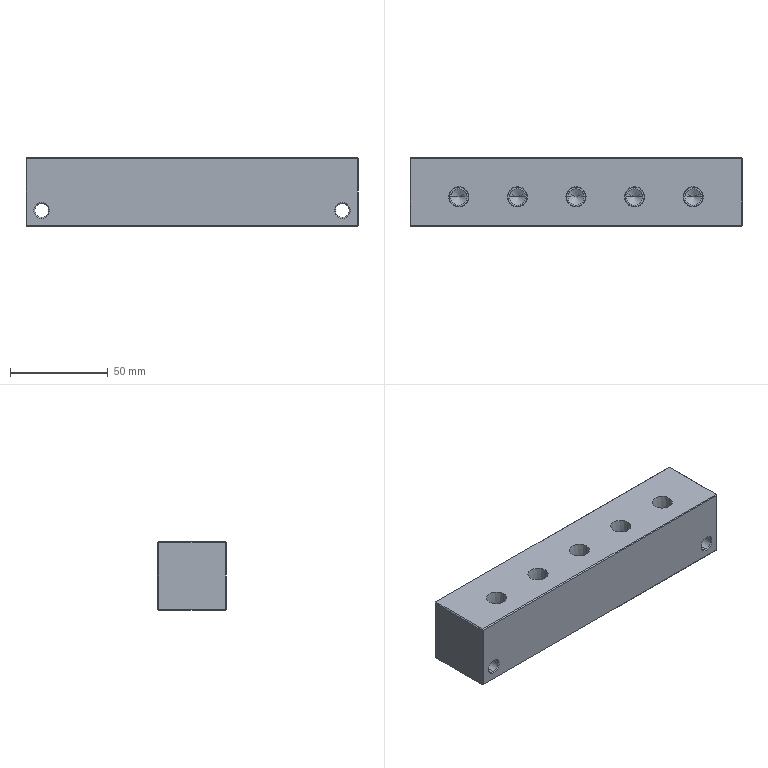Part | STEP file | OP10-135_junction block (E) | 1 solid | 109 faces | box 170 x 35 x 35 mm | volume 190983 mm3 | cone 38 | plane 38 | cylinder 33 | commonest cylinder face diameters 8.433 x25 7 x4 11 x4